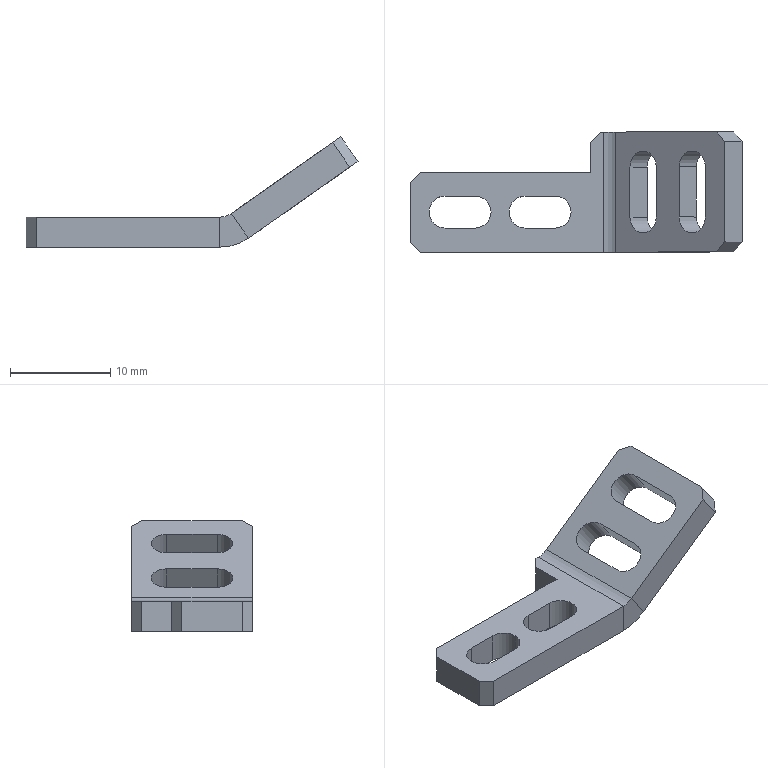Part | SolidWorks | features ICE 2, Chamfer 1, Cut 1, EdgeFlange 1, FlatPattern 1, SMBaseFlange 1, SheetMetal 1 | 1 solid | 39 faces | box 33.189 x 12 x 11.03 mm | volume 781.956 mm3 | plane 27 | cylinder 12 | commonest cylinder face diameters 3.2 x10 4 x1 10 x1
STEP:
#1=CARTESIAN_POINT('',(6.1,-2.,-3.));
#2=VERTEX_POINT('',#1);
#3=CARTESIAN_POINT('',(4.5,-0.4,-3.));
#4=VERTEX_POINT('',#3);
#5=CARTESIAN_POINT('',(4.5,-2.,-3.));
#6=DIRECTION('',(0.,0.,1.));
#7=DIRECTION('',(1.,0.,0.));
#8=AXIS2_PLACEMENT_3D('',#5,#6,#7);
#9=CIRCLE('',#8,1.6);
#10=EDGE_CURVE('',#2,#4,#9,.T.);
#11=ORIENTED_EDGE('',*,*,#10,.F.);
#12=CARTESIAN_POINT('',(6.1,-2.,0.));
#13=VERTEX_POINT('',#12);
#14=CARTESIAN_POINT('',(6.1,-2.,-3.));
#15=DIRECTION('',(0.,0.,1.));
#16=VECTOR('',#15,1000.);
#17=LINE('',#14,#16);
#18=EDGE_CURVE('',#2,#13,#17,.T.);
#19=ORIENTED_EDGE('',*,*,#18,.T.);
#20=CARTESIAN_POINT('',(4.5,-0.4,0.));
#21=VERTEX_POINT('',#20);
#22=CARTESIAN_POINT('',(4.5,-2.,0.));
#23=DIRECTION('',(0.,0.,1.));
#24=DIRECTION('',(1.,0.,0.));
#25=AXIS2_PLACEMENT_3D('',#22,#23,#24);
#26=CIRCLE('',#25,1.6);
#27=EDGE_CURVE('',#13,#21,#26,.T.);
#28=ORIENTED_EDGE('',*,*,#27,.T.);
#29=CARTESIAN_POINT('',(4.5,-0.4,-3.));
#30=DIRECTION('',(0.,0.,1.));
#31=VECTOR('',#30,1000.);
#32=LINE('',#29,#31);
#33=EDGE_CURVE('',#4,#21,#32,.T.);
#34=ORIENTED_EDGE('',*,*,#33,.F.);
#35=EDGE_LOOP('',(#11,#19,#28,#34));
#36=FACE_OUTER_BOUND('',#35,.T.);
#37=CARTESIAN_POINT('',(4.5,-2.,-3.));
#38=DIRECTION('',(0.,0.,1.));
#39=DIRECTION('',(1.,0.,0.));
#40=AXIS2_PLACEMENT_3D('',#37,#38,#39);
#41=CYLINDRICAL_SURFACE('',#40,1.6);
#42=ADVANCED_FACE('',(#36),#41,.F.);
#43=CARTESIAN_POINT('',(-1.9,-2.,-3.));
#44=VERTEX_POINT('',#43);
#45=CARTESIAN_POINT('',(-3.5,-0.4,-3.));
#46=VERTEX_POINT('',#45);
#47=CARTESIAN_POINT('',(-3.5,-2.,-3.));
#48=DIRECTION('',(0.,0.,1.));
#49=DIRECTION('',(1.,0.,0.));
#50=AXIS2_PLACEMENT_3D('',#47,#48,#49);
#51=CIRCLE('',#50,1.6);
#52=EDGE_CURVE('',#44,#46,#51,.T.);
#53=ORIENTED_EDGE('',*,*,#52,.F.);
#54=CARTESIAN_POINT('',(-1.9,-2.,0.));
#55=VERTEX_POINT('',#54);
#56=CARTESIAN_POINT('',(-1.9,-2.,-3.));
#57=DIRECTION('',(0.,0.,1.));
#58=VECTOR('',#57,1000.);
#59=LINE('',#56,#58);
#60=EDGE_CURVE('',#44,#55,#59,.T.);
#61=ORIENTED_EDGE('',*,*,#60,.T.);
#62=CARTESIAN_POINT('',(-3.5,-0.4,0.));
#63=VERTEX_POINT('',#62);
#64=CARTESIAN_POINT('',(-3.5,-2.,0.));
#65=DIRECTION('',(0.,0.,1.));
#66=DIRECTION('',(1.,0.,0.));
#67=AXIS2_PLACEMENT_3D('',#64,#65,#66);
#68=CIRCLE('',#67,1.6);
#69=EDGE_CURVE('',#55,#63,#68,.T.);
#70=ORIENTED_EDGE('',*,*,#69,.T.);
#71=CARTESIAN_POINT('',(-3.5,-0.4,-3.));
#72=DIRECTION('',(0.,0.,1.));
#73=VECTOR('',#72,1000.);
#74=LINE('',#71,#73);
#75=EDGE_CURVE('',#46,#63,#74,.T.);
#76=ORIENTED_EDGE('',*,*,#75,.F.);
#77=EDGE_LOOP('',(#53,#61,#70,#76));
#78=FACE_OUTER_BOUND('',#77,.T.);
#79=CARTESIAN_POINT('',(-3.5,-2.,-3.));
#80=DIRECTION('',(0.,0.,1.));
#81=DIRECTION('',(1.,0.,0.));
#82=AXIS2_PLACEMENT_3D('',#79,#80,#81);
#83=CYLINDRICAL_SURFACE('',#82,1.6);
#84=ADVANCED_FACE('',(#78),#83,.F.);
#85=CARTESIAN_POINT('',(9.369,6.,-3.));
#86=VERTEX_POINT('',#85);
#87=CARTESIAN_POINT('',(9.,6.,-3.));
#88=VERTEX_POINT('',#87);
#89=CARTESIAN_POINT('',(-10.,6.,-3.));
#90=DIRECTION('',(-1.,0.,0.));
#91=VECTOR('',#90,1000.);
#92=LINE('',#89,#91);
#93=EDGE_CURVE('',#86,#88,#92,.T.);
#94=ORIENTED_EDGE('',*,*,#93,.T.);
#95=CARTESIAN_POINT('',(9.,6.,0.));
#96=VERTEX_POINT('',#95);
#97=CARTESIAN_POINT('',(9.,6.,0.));
#98=DIRECTION('',(0.,0.,1.));
#99=VECTOR('',#98,1000.);
#100=LINE('',#97,#99);
#101=EDGE_CURVE('',#88,#96,#100,.T.);
#102=ORIENTED_EDGE('',*,*,#101,.T.);
#103=CARTESIAN_POINT('',(9.369,6.,0.));
#104=VERTEX_POINT('',#103);
#105=CARTESIAN_POINT('',(-10.,6.,0.));
#106=DIRECTION('',(-1.,0.,0.));
#107=VECTOR('',#106,1000.);
#108=LINE('',#105,#107);
#109=EDGE_CURVE('',#104,#96,#108,.T.);
#110=ORIENTED_EDGE('',*,*,#109,.F.);
#111=CARTESIAN_POINT('',(9.369,6.,0.));
#112=DIRECTION('',(0.,0.,-1.));
#113=VECTOR('',#112,1000.);
#114=LINE('',#111,#113);
#115=EDGE_CURVE('',#104,#86,#114,.T.);
#116=ORIENTED_EDGE('',*,*,#115,.T.);
#117=EDGE_LOOP('',(#94,#102,#110,#116));
#118=FACE_OUTER_BOUND('',#117,.T.);
#119=CARTESIAN_POINT('',(-10.,6.,-3.));
#120=DIRECTION('',(0.,1.,0.));
#121=DIRECTION('',(0.,0.,1.));
#122=AXIS2_PLACEMENT_3D('',#119,#120,#121);
#123=PLANE('',#122);
#124=ADVANCED_FACE('',(#118),#123,.T.);
#125=CARTESIAN_POINT('',(1.5,-0.4,-3.));
#126=VERTEX_POINT('',#125);
#127=CARTESIAN_POINT('',(1.5,-0.4,-3.));
#128=DIRECTION('',(-1.,0.,0.));
#129=VECTOR('',#128,1000.);
#130=LINE('',#127,#129);
#131=EDGE_CURVE('',#4,#126,#130,.T.);
#132=ORIENTED_EDGE('',*,*,#131,.T.);
#133=CARTESIAN_POINT('',(1.5,-3.6,-3.));
#134=VERTEX_POINT('',#133);
#135=CARTESIAN_POINT('',(1.5,-2.,-3.));
#136=DIRECTION('',(0.,0.,1.));
#137=DIRECTION('',(1.,0.,0.));
#138=AXIS2_PLACEMENT_3D('',#135,#136,#137);
#139=CIRCLE('',#138,1.6);
#140=EDGE_CURVE('',#126,#134,#139,.T.);
#141=ORIENTED_EDGE('',*,*,#140,.T.);
#142=CARTESIAN_POINT('',(4.5,-3.6,-3.));
#143=VERTEX_POINT('',#142);
#144=CARTESIAN_POINT('',(1.5,-3.6,-3.));
#145=DIRECTION('',(1.,0.,0.));
#146=VECTOR('',#145,1000.);
#147=LINE('',#144,#146);
#148=EDGE_CURVE('',#134,#143,#147,.T.);
#149=ORIENTED_EDGE('',*,*,#148,.T.);
#150=CARTESIAN_POINT('',(4.5,-2.,-3.));
#151=DIRECTION('',(0.,0.,1.));
#152=DIRECTION('',(1.,0.,0.));
#153=AXIS2_PLACEMENT_3D('',#150,#151,#152);
#154=CIRCLE('',#153,1.6);
#155=EDGE_CURVE('',#143,#2,#154,.T.);
#156=ORIENTED_EDGE('',*,*,#155,.T.);
#157=ORIENTED_EDGE('',*,*,#10,.T.);
#158=EDGE_LOOP('',(#132,#141,#149,#156,#157));
#159=FACE_BOUND('',#158,.T.);
#160=CARTESIAN_POINT('',(-6.5,-0.4,-3.));
#161=VERTEX_POINT('',#160);
#162=CARTESIAN_POINT('',(-6.5,-0.4,-3.));
#163=DIRECTION('',(-1.,0.,0.));
#164=VECTOR('',#163,1000.);
#165=LINE('',#162,#164);
#166=EDGE_CURVE('',#46,#161,#165,.T.);
#167=ORIENTED_EDGE('',*,*,#166,.T.);
#168=CARTESIAN_POINT('',(-6.5,-3.6,-3.));
#169=VERTEX_POINT('',#168);
#170=CARTESIAN_POINT('',(-6.5,-2.,-3.));
#171=DIRECTION('',(0.,0.,1.));
#172=DIRECTION('',(1.,0.,0.));
#173=AXIS2_PLACEMENT_3D('',#170,#171,#172);
#174=CIRCLE('',#173,1.6);
#175=EDGE_CURVE('',#161,#169,#174,.T.);
#176=ORIENTED_EDGE('',*,*,#175,.T.);
#177=CARTESIAN_POINT('',(-3.5,-3.6,-3.));
#178=VERTEX_POINT('',#177);
#179=CARTESIAN_POINT('',(-6.5,-3.6,-3.));
#180=DIRECTION('',(1.,0.,0.));
#181=VECTOR('',#180,1000.);
#182=LINE('',#179,#181);
#183=EDGE_CURVE('',#169,#178,#182,.T.);
#184=ORIENTED_EDGE('',*,*,#183,.T.);
#185=CARTESIAN_POINT('',(-3.5,-2.,-3.));
#186=DIRECTION('',(0.,0.,1.));
#187=DIRECTION('',(1.,0.,0.));
#188=AXIS2_PLACEMENT_3D('',#185,#186,#187);
#189=CIRCLE('',#188,1.6);
#190=EDGE_CURVE('',#178,#44,#189,.T.);
#191=ORIENTED_EDGE('',*,*,#190,.T.);
#192=ORIENTED_EDGE('',*,*,#52,.T.);
#193=EDGE_LOOP('',(#167,#176,#184,#191,#192));
#194=FACE_BOUND('',#193,.T.);
#195=CARTESIAN_POINT('',(8.,2.,-3.));
#196=VERTEX_POINT('',#195);
#197=CARTESIAN_POINT('',(8.,5.,-3.));
#198=VERTEX_POINT('',#197);
#199=CARTESIAN_POINT('',(8.,6.,-3.));
#200=DIRECTION('',(0.,1.,0.));
#201=VECTOR('',#200,1000.);
#202=LINE('',#199,#201);
#203=EDGE_CURVE('',#196,#198,#202,.T.);
#204=ORIENTED_EDGE('',*,*,#203,.T.);
#205=CARTESIAN_POINT('',(9.,6.,-3.));
#206=DIRECTION('',(0.7071,0.7071,0.));
#207=VECTOR('',#206,1000.);
#208=LINE('',#205,#207);
#209=EDGE_CURVE('',#198,#88,#208,.T.);
#210=ORIENTED_EDGE('',*,*,#209,.T.);
#211=ORIENTED_EDGE('',*,*,#93,.F.);
#212=CARTESIAN_POINT('',(9.369,-6.,-3.));
#213=VERTEX_POINT('',#212);
#214=CARTESIAN_POINT('',(9.369,6.,-3.));
#215=DIRECTION('',(0.,-1.,0.));
#216=VECTOR('',#215,1000.);
#217=LINE('',#214,#216);
#218=EDGE_CURVE('',#86,#213,#217,.T.);
#219=ORIENTED_EDGE('',*,*,#218,.T.);
#220=CARTESIAN_POINT('',(-9.,-6.,-3.));
#221=VERTEX_POINT('',#220);
#222=CARTESIAN_POINT('',(-10.,-6.,-3.));
#223=DIRECTION('',(1.,0.,0.));
#224=VECTOR('',#223,1000.);
#225=LINE('',#222,#224);
#226=EDGE_CURVE('',#221,#213,#225,.T.);
#227=ORIENTED_EDGE('',*,*,#226,.F.);
#228=CARTESIAN_POINT('',(-10.,-5.,-3.));
#229=VERTEX_POINT('',#228);
#230=CARTESIAN_POINT('',(-10.,-5.,-3.));
#231=DIRECTION('',(-0.7071,0.7071,0.));
#232=VECTOR('',#231,1000.);
#233=LINE('',#230,#232);
#234=EDGE_CURVE('',#221,#229,#233,.T.);
#235=ORIENTED_EDGE('',*,*,#234,.T.);
#236=CARTESIAN_POINT('',(-10.,1.,-3.));
#237=VERTEX_POINT('',#236);
#238=CARTESIAN_POINT('',(-10.,6.,-3.));
#239=DIRECTION('',(0.,-1.,0.));
#240=VECTOR('',#239,1000.);
#241=LINE('',#238,#240);
#242=EDGE_CURVE('',#237,#229,#241,.T.);
#243=ORIENTED_EDGE('',*,*,#242,.F.);
#244=CARTESIAN_POINT('',(-9.,2.,-3.));
#245=VERTEX_POINT('',#244);
#246=CARTESIAN_POINT('',(-9.,2.,-3.));
#247=DIRECTION('',(0.7071,0.7071,0.));
#248=VECTOR('',#247,1000.);
#249=LINE('',#246,#248);
#250=EDGE_CURVE('',#237,#245,#249,.T.);
#251=ORIENTED_EDGE('',*,*,#250,.T.);
#252=CARTESIAN_POINT('',(-10.,2.,-3.));
#253=DIRECTION('',(1.,0.,0.));
#254=VECTOR('',#253,1000.);
#255=LINE('',#252,#254);
#256=EDGE_CURVE('',#245,#196,#255,.T.);
#257=ORIENTED_EDGE('',*,*,#256,.T.);
#258=EDGE_LOOP('',(#204,#210,#211,#219,#227,#235,#243,#251,#257));
#259=FACE_OUTER_BOUND('',#258,.T.);
#260=CARTESIAN_POINT('',(0.,0.,-3.));
#261=DIRECTION('',(0.,0.,1.));
#262=DIRECTION('',(1.,0.,0.));
#263=AXIS2_PLACEMENT_3D('',#260,#261,#262);
#264=PLANE('',#263);
#265=ADVANCED_FACE('',(#159,#194,#259),#264,.F.);
#266=ORIENTED_EDGE('',*,*,#109,.T.);
#267=CARTESIAN_POINT('',(8.,5.,0.));
#268=VERTEX_POINT('',#267);
#269=CARTESIAN_POINT('',(1.5,-1.5,0.));
#270=DIRECTION('',(-0.7071,-0.7071,0.));
#271=VECTOR('',#270,1000.);
#272=LINE('',#269,#271);
#273=EDGE_CURVE('',#96,#268,#272,.T.);
#274=ORIENTED_EDGE('',*,*,#273,.T.);
#275=CARTESIAN_POINT('',(8.,2.,0.));
#276=VERTEX_POINT('',#275);
#277=CARTESIAN_POINT('',(8.,6.,0.));
#278=DIRECTION('',(0.,1.,0.));
#279=VECTOR('',#278,1000.);
#280=LINE('',#277,#279);
#281=EDGE_CURVE('',#276,#268,#280,.T.);
#282=ORIENTED_EDGE('',*,*,#281,.F.);
#283=CARTESIAN_POINT('',(-9.,2.,0.));
#284=VERTEX_POINT('',#283);
#285=CARTESIAN_POINT('',(-10.,2.,0.));
#286=DIRECTION('',(1.,0.,0.));
#287=VECTOR('',#286,1000.);
#288=LINE('',#285,#287);
#289=EDGE_CURVE('',#284,#276,#288,.T.);
#290=ORIENTED_EDGE('',*,*,#289,.F.);
#291=CARTESIAN_POINT('',(-10.,1.,0.));
#292=VERTEX_POINT('',#291);
#293=CARTESIAN_POINT('',(-5.5,5.5,0.));
#294=DIRECTION('',(-0.7071,-0.7071,0.));
#295=VECTOR('',#294,1000.);
#296=LINE('',#293,#295);
#297=EDGE_CURVE('',#284,#292,#296,.T.);
#298=ORIENTED_EDGE('',*,*,#297,.T.);
#299=CARTESIAN_POINT('',(-10.,-5.,0.));
#300=VERTEX_POINT('',#299);
#301=CARTESIAN_POINT('',(-10.,6.,0.));
#302=DIRECTION('',(0.,-1.,0.));
#303=VECTOR('',#302,1000.);
#304=LINE('',#301,#303);
#305=EDGE_CURVE('',#292,#300,#304,.T.);
#306=ORIENTED_EDGE('',*,*,#305,.T.);
#307=CARTESIAN_POINT('',(-9.,-6.,0.));
#308=VERTEX_POINT('',#307);
#309=CARTESIAN_POINT('',(-7.5,-7.5,0.));
#310=DIRECTION('',(0.7071,-0.7071,0.));
#311=VECTOR('',#310,1000.);
#312=LINE('',#309,#311);
#313=EDGE_CURVE('',#300,#308,#312,.T.);
#314=ORIENTED_EDGE('',*,*,#313,.T.);
#315=CARTESIAN_POINT('',(9.369,-6.,0.));
#316=VERTEX_POINT('',#315);
#317=CARTESIAN_POINT('',(-10.,-6.,0.));
#318=DIRECTION('',(1.,0.,0.));
#319=VECTOR('',#318,1000.);
#320=LINE('',#317,#319);
#321=EDGE_CURVE('',#308,#316,#320,.T.);
#322=ORIENTED_EDGE('',*,*,#321,.T.);
#323=CARTESIAN_POINT('',(9.369,6.,0.));
#324=DIRECTION('',(0.,-1.,0.));
#325=VECTOR('',#324,1000.);
#326=LINE('',#323,#325);
#327=EDGE_CURVE('',#104,#316,#326,.T.);
#328=ORIENTED_EDGE('',*,*,#327,.F.);
#329=EDGE_LOOP('',(#266,#274,#282,#290,#298,#306,#314,#322,#328));
#330=FACE_OUTER_BOUND('',#329,.T.);
#331=CARTESIAN_POINT('',(1.5,-0.4,0.));
#332=VERTEX_POINT('',#331);
#333=CARTESIAN_POINT('',(1.5,-3.6,0.));
#334=VERTEX_POINT('',#333);
#335=CARTESIAN_POINT('',(1.5,-2.,0.));
#336=DIRECTION('',(0.,0.,1.));
#337=DIRECTION('',(1.,0.,0.));
#338=AXIS2_PLACEMENT_3D('',#335,#336,#337);
#339=CIRCLE('',#338,1.6);
#340=EDGE_CURVE('',#332,#334,#339,.T.);
#341=ORIENTED_EDGE('',*,*,#340,.F.);
#342=CARTESIAN_POINT('',(1.5,-0.4,0.));
#343=DIRECTION('',(-1.,0.,0.));
#344=VECTOR('',#343,1000.);
#345=LINE('',#342,#344);
#346=EDGE_CURVE('',#21,#332,#345,.T.);
#347=ORIENTED_EDGE('',*,*,#346,.F.);
#348=ORIENTED_EDGE('',*,*,#27,.F.);
#349=CARTESIAN_POINT('',(4.5,-3.6,0.));
#350=VERTEX_POINT('',#349);
#351=CARTESIAN_POINT('',(4.5,-2.,0.));
#352=DIRECTION('',(0.,0.,1.));
#353=DIRECTION('',(1.,0.,0.));
#354=AXIS2_PLACEMENT_3D('',#351,#352,#353);
#355=CIRCLE('',#354,1.6);
#356=EDGE_CURVE('',#350,#13,#355,.T.);
#357=ORIENTED_EDGE('',*,*,#356,.F.);
#358=CARTESIAN_POINT('',(1.5,-3.6,0.));
#359=DIRECTION('',(1.,0.,0.));
#360=VECTOR('',#359,1000.);
#361=LINE('',#358,#360);
#362=EDGE_CURVE('',#334,#350,#361,.T.);
#363=ORIENTED_EDGE('',*,*,#362,.F.);
#364=EDGE_LOOP('',(#341,#347,#348,#357,#363));
#365=FACE_BOUND('',#364,.T.);
#366=CARTESIAN_POINT('',(-6.5,-0.4,0.));
#367=VERTEX_POINT('',#366);
#368=CARTESIAN_POINT('',(-6.5,-3.6,0.));
#369=VERTEX_POINT('',#368);
#370=CARTESIAN_POINT('',(-6.5,-2.,0.));
#371=DIRECTION('',(0.,0.,1.));
#372=DIRECTION('',(1.,0.,0.));
#373=AXIS2_PLACEMENT_3D('',#370,#371,#372);
#374=CIRCLE('',#373,1.6);
#375=EDGE_CURVE('',#367,#369,#374,.T.);
#376=ORIENTED_EDGE('',*,*,#375,.F.);
#377=CARTESIAN_POINT('',(-6.5,-0.4,0.));
#378=DIRECTION('',(-1.,0.,0.));
#379=VECTOR('',#378,1000.);
#380=LINE('',#377,#379);
#381=EDGE_CURVE('',#63,#367,#380,.T.);
#382=ORIENTED_EDGE('',*,*,#381,.F.);
#383=ORIENTED_EDGE('',*,*,#69,.F.);
#384=CARTESIAN_POINT('',(-3.5,-3.6,0.));
#385=VERTEX_POINT('',#384);
#386=CARTESIAN_POINT('',(-3.5,-2.,0.));
#387=DIRECTION('',(0.,0.,1.));
#388=DIRECTION('',(1.,0.,0.));
#389=AXIS2_PLACEMENT_3D('',#386,#387,#388);
#390=CIRCLE('',#389,1.6);
#391=EDGE_CURVE('',#385,#55,#390,.T.);
#392=ORIENTED_EDGE('',*,*,#391,.F.);
#393=CARTESIAN_POINT('',(-6.5,-3.6,0.));
#394=DIRECTION('',(1.,0.,0.));
#395=VECTOR('',#394,1000.);
#396=LINE('',#393,#395);
#397=EDGE_CURVE('',#369,#385,#396,.T.);
#398=ORIENTED_EDGE('',*,*,#397,.F.);
#399=EDGE_LOOP('',(#376,#382,#383,#392,#398));
#400=FACE_BOUND('',#399,.T.);
#401=CARTESIAN_POINT('',(0.,0.,0.));
#402=DIRECTION('',(0.,0.,1.));
#403=DIRECTION('',(1.,0.,0.));
#404=AXIS2_PLACEMENT_3D('',#401,#402,#403);
#405=PLANE('',#404);
#406=ADVANCED_FACE('',(#330,#365,#400),#405,.T.);
#407=ORIENTED_EDGE('',*,*,#321,.F.);
#408=CARTESIAN_POINT('',(-9.,-6.,-3.));
#409=DIRECTION('',(0.,0.,-1.));
#410=VECTOR('',#409,1000.);
#411=LINE('',#408,#410);
#412=EDGE_CURVE('',#308,#221,#411,.T.);
#413=ORIENTED_EDGE('',*,*,#412,.T.);
#414=ORIENTED_EDGE('',*,*,#226,.T.);
#415=CARTESIAN_POINT('',(9.369,-6.,0.));
#416=DIRECTION('',(0.,0.,-1.));
#417=VECTOR('',#416,1000.);
#418=LINE('',#415,#417);
#419=EDGE_CURVE('',#316,#213,#418,.T.);
#420=ORIENTED_EDGE('',*,*,#419,.F.);
#421=EDGE_LOOP('',(#407,#413,#414,#420));
#422=FACE_OUTER_BOUND('',#421,.T.);
#423=CARTESIAN_POINT('',(-10.,-6.,-3.));
#424=DIRECTION('',(0.,-1.,0.));
#425=DIRECTION('',(0.,0.,-1.));
#426=AXIS2_PLACEMENT_3D('',#423,#424,#425);
#427=PLANE('',#426);
#428=ADVANCED_FACE('',(#422),#427,.T.);
#429=ORIENTED_EDGE('',*,*,#242,.T.);
#430=CARTESIAN_POINT('',(-10.,-5.,-3.));
#431=DIRECTION('',(0.,0.,1.));
#432=VECTOR('',#431,1000.);
#433=LINE('',#430,#432);
#434=EDGE_CURVE('',#229,#300,#433,.T.);
#435=ORIENTED_EDGE('',*,*,#434,.T.);
#436=ORIENTED_EDGE('',*,*,#305,.F.);
#437=CARTESIAN_POINT('',(-10.,1.,-3.));
#438=DIRECTION('',(0.,0.,-1.));
#439=VECTOR('',#438,1000.);
#440=LINE('',#437,#439);
#441=EDGE_CURVE('',#292,#237,#440,.T.);
#442=ORIENTED_EDGE('',*,*,#441,.T.);
#443=EDGE_LOOP('',(#429,#435,#436,#442));
#444=FACE_OUTER_BOUND('',#443,.T.);
#445=CARTESIAN_POINT('',(-10.,6.,-3.));
#446=DIRECTION('',(-1.,0.,0.));
#447=DIRECTION('',(0.,0.,1.));
#448=AXIS2_PLACEMENT_3D('',#445,#446,#447);
#449=PLANE('',#448);
#450=ADVANCED_FACE('',(#444),#449,.T.);
#451=CARTESIAN_POINT('',(10.517,-6.,0.3617));
#452=VERTEX_POINT('',#451);
#453=CARTESIAN_POINT('',(12.237,-6.,-2.096));
#454=VERTEX_POINT('',#453);
#455=CARTESIAN_POINT('',(10.517,-6.,0.3617));
#456=DIRECTION('',(0.5736,0.,-0.8192));
#457=VECTOR('',#456,1000.);
#458=LINE('',#455,#457);
#459=EDGE_CURVE('',#452,#454,#458,.T.);
#460=ORIENTED_EDGE('',*,*,#459,.F.);
#461=CARTESIAN_POINT('',(9.369,-6.,2.));
#462=DIRECTION('',(0.,-1.,0.));
#463=DIRECTION('',(0.,0.,1.));
#464=AXIS2_PLACEMENT_3D('',#461,#462,#463);
#465=CIRCLE('',#464,2.);
#466=EDGE_CURVE('',#316,#452,#465,.T.);
#467=ORIENTED_EDGE('',*,*,#466,.F.);
#468=ORIENTED_EDGE('',*,*,#419,.T.);
#469=CARTESIAN_POINT('',(9.369,-6.,2.));
#470=DIRECTION('',(0.,-1.,0.));
#471=DIRECTION('',(0.,0.,1.));
#472=AXIS2_PLACEMENT_3D('',#469,#470,#471);
#473=CIRCLE('',#472,5.);
#474=EDGE_CURVE('',#213,#454,#473,.T.);
#475=ORIENTED_EDGE('',*,*,#474,.T.);
#476=EDGE_LOOP('',(#460,#467,#468,#475));
#477=FACE_OUTER_BOUND('',#476,.T.);
#478=CARTESIAN_POINT('',(9.369,-6.,2.));
#479=DIRECTION('',(0.,-1.,0.));
#480=DIRECTION('',(0.,0.,-1.));
#481=AXIS2_PLACEMENT_3D('',#478,#479,#480);
#482=PLANE('',#481);
#483=ADVANCED_FACE('',(#477),#482,.T.);
#484=CARTESIAN_POINT('',(10.517,6.,0.3617));
#485=VERTEX_POINT('',#484);
#486=CARTESIAN_POINT('',(9.369,6.,2.));
#487=DIRECTION('',(0.,1.,0.));
#488=DIRECTION('',(0.,0.,1.));
#489=AXIS2_PLACEMENT_3D('',#486,#487,#488);
#490=CIRCLE('',#489,2.);
#491=EDGE_CURVE('',#485,#104,#490,.T.);
#492=ORIENTED_EDGE('',*,*,#491,.F.);
#493=CARTESIAN_POINT('',(12.237,6.,-2.096));
#494=VERTEX_POINT('',#493);
#495=CARTESIAN_POINT('',(10.517,6.,0.3617));
#496=DIRECTION('',(0.5736,0.,-0.8192));
#497=VECTOR('',#496,1000.);
#498=LINE('',#495,#497);
#499=EDGE_CURVE('',#485,#494,#498,.T.);
#500=ORIENTED_EDGE('',*,*,#499,.T.);
#501=CARTESIAN_POINT('',(9.369,6.,2.));
#502=DIRECTION('',(0.,1.,0.));
#503=DIRECTION('',(0.,0.,1.));
#504=AXIS2_PLACEMENT_3D('',#501,#502,#503);
#505=CIRCLE('',#504,5.);
#506=EDGE_CURVE('',#494,#86,#505,.T.);
#507=ORIENTED_EDGE('',*,*,#506,.T.);
#508=ORIENTED_EDGE('',*,*,#115,.F.);
#509=EDGE_LOOP('',(#492,#500,#507,#508));
#510=FACE_OUTER_BOUND('',#509,.T.);
#511=CARTESIAN_POINT('',(9.369,6.,2.));
#512=DIRECTION('',(0.,-1.,0.));
#513=DIRECTION('',(0.,0.,-1.));
#514=AXIS2_PLACEMENT_3D('',#511,#512,#513);
#515=PLANE('',#514);
#516=ADVANCED_FACE('',(#510),#515,.F.);
#517=ORIENTED_EDGE('',*,*,#218,.F.);
#518=ORIENTED_EDGE('',*,*,#506,.F.);
#519=CARTESIAN_POINT('',(12.237,0.,-2.096));
#520=DIRECTION('',(0.,1.,0.));
#521=VECTOR('',#520,1000.);
#522=LINE('',#519,#521);
#523=EDGE_CURVE('',#454,#494,#522,.T.);
#524=ORIENTED_EDGE('',*,*,#523,.F.);
#525=ORIENTED_EDGE('',*,*,#474,.F.);
#526=EDGE_LOOP('',(#517,#518,#524,#525));
#527=FACE_OUTER_BOUND('',#526,.T.);
#528=CARTESIAN_POINT('',(9.369,6.,2.));
#529=DIRECTION('',(0.,1.,0.));
#530=DIRECTION('',(0.5736,0.,-0.8192));
#531=AXIS2_PLACEMENT_3D('',#528,#529,#530);
#532=CYLINDRICAL_SURFACE('',#531,5.);
#533=ADVANCED_FACE('',(#527),#532,.T.);
#534=ORIENTED_EDGE('',*,*,#327,.T.);
#535=ORIENTED_EDGE('',*,*,#466,.T.);
#536=CARTESIAN_POINT('',(10.517,-6.,0.3617));
#537=DIRECTION('',(0.,1.,0.));
#538=VECTOR('',#537,1000.);
#539=LINE('',#536,#538);
#540=EDGE_CURVE('',#452,#485,#539,.T.);
#541=ORIENTED_EDGE('',*,*,#540,.T.);
#542=ORIENTED_EDGE('',*,*,#491,.T.);
#543=EDGE_LOOP('',(#534,#535,#541,#542));
#544=FACE_OUTER_BOUND('',#543,.T.);
#545=CARTESIAN_POINT('',(9.369,6.,2.));
#546=DIRECTION('',(0.,1.,0.));
#547=DIRECTION('',(0.5736,0.,-0.8192));
#548=AXIS2_PLACEMENT_3D('',#545,#546,#547);
#549=CYLINDRICAL_SURFACE('',#548,2.);
#550=ADVANCED_FACE('',(#544),#549,.F.);
#551=CARTESIAN_POINT('',(20.649,6.,7.456));
#552=VERTEX_POINT('',#551);
#553=CARTESIAN_POINT('',(10.,6.,0.));
#554=DIRECTION('',(-0.8192,0.,-0.5736));
#555=VECTOR('',#554,1000.);
#556=LINE('',#553,#555);
#557=EDGE_CURVE('',#552,#485,#556,.T.);
#558=ORIENTED_EDGE('',*,*,#557,.F.);
#559=CARTESIAN_POINT('',(22.37,6.,4.999));
#560=VERTEX_POINT('',#559);
#561=CARTESIAN_POINT('',(22.37,6.,4.999));
#562=DIRECTION('',(0.5736,0.,-0.8192));
#563=VECTOR('',#562,1000.);
#564=LINE('',#561,#563);
#565=EDGE_CURVE('',#552,#560,#564,.T.);
#566=ORIENTED_EDGE('',*,*,#565,.T.);
#567=CARTESIAN_POINT('',(11.721,6.,-2.457));
#568=DIRECTION('',(-0.8192,0.,-0.5736));
#569=VECTOR('',#568,1000.);
#570=LINE('',#567,#569);
#571=EDGE_CURVE('',#560,#494,#570,.T.);
#572=ORIENTED_EDGE('',*,*,#571,.T.);
#573=ORIENTED_EDGE('',*,*,#499,.F.);
#574=EDGE_LOOP('',(#558,#566,#572,#573));
#575=FACE_OUTER_BOUND('',#574,.T.);
#576=CARTESIAN_POINT('',(11.721,6.,-2.457));
#577=DIRECTION('',(0.,1.,0.));
#578=DIRECTION('',(-1.,0.,0.));
#579=AXIS2_PLACEMENT_3D('',#576,#577,#578);
#580=PLANE('',#579);
#581=ADVANCED_FACE('',(#575),#580,.T.);
#582=CARTESIAN_POINT('',(22.37,-6.,4.999));
#583=VERTEX_POINT('',#582);
#584=CARTESIAN_POINT('',(23.189,-6.,5.573));
#585=DIRECTION('',(0.8192,0.,0.5736));
#586=VECTOR('',#585,1000.);
#587=LINE('',#584,#586);
#588=EDGE_CURVE('',#454,#583,#587,.T.);
#589=ORIENTED_EDGE('',*,*,#588,.T.);
#590=CARTESIAN_POINT('',(20.649,-6.,7.456));
#591=VERTEX_POINT('',#590);
#592=CARTESIAN_POINT('',(22.37,-6.,4.999));
#593=DIRECTION('',(-0.5736,0.,0.8192));
#594=VECTOR('',#593,1000.);
#595=LINE('',#592,#594);
#596=EDGE_CURVE('',#583,#591,#595,.T.);
#597=ORIENTED_EDGE('',*,*,#596,.T.);
#598=CARTESIAN_POINT('',(21.468,-6.,8.03));
#599=DIRECTION('',(0.8192,0.,0.5736));
#600=VECTOR('',#599,1000.);
#601=LINE('',#598,#600);
#602=EDGE_CURVE('',#452,#591,#601,.T.);
#603=ORIENTED_EDGE('',*,*,#602,.F.);
#604=ORIENTED_EDGE('',*,*,#459,.T.);
#605=EDGE_LOOP('',(#589,#597,#603,#604));
#606=FACE_OUTER_BOUND('',#605,.T.);
#607=CARTESIAN_POINT('',(23.189,-6.,5.573));
#608=DIRECTION('',(0.,-1.,0.));
#609=DIRECTION('',(1.,0.,0.));
#610=AXIS2_PLACEMENT_3D('',#607,#608,#609);
#611=PLANE('',#610);
#612=ADVANCED_FACE('',(#606),#611,.T.);
#613=CARTESIAN_POINT('',(18.625,2.5,2.377));
#614=VERTEX_POINT('',#613);
#615=CARTESIAN_POINT('',(21.246,2.5,4.212));
#616=VERTEX_POINT('',#615);
#617=CARTESIAN_POINT('',(19.935,2.5,3.294));
#618=DIRECTION('',(0.5736,0.,-0.8192));
#619=DIRECTION('',(-0.8192,0.,-0.5736));
#620=AXIS2_PLACEMENT_3D('',#617,#618,#619);
#621=CIRCLE('',#620,1.6);
#622=EDGE_CURVE('',#614,#616,#621,.T.);
#623=ORIENTED_EDGE('',*,*,#622,.F.);
#624=CARTESIAN_POINT('',(18.625,-2.5,2.377));
#625=VERTEX_POINT('',#624);
#626=CARTESIAN_POINT('',(18.625,0.,2.377));
#627=DIRECTION('',(0.,1.,0.));
#628=VECTOR('',#627,1000.);
#629=LINE('',#626,#628);
#630=EDGE_CURVE('',#625,#614,#629,.T.);
#631=ORIENTED_EDGE('',*,*,#630,.F.);
#632=CARTESIAN_POINT('',(21.246,-2.5,4.212));
#633=VERTEX_POINT('',#632);
#634=CARTESIAN_POINT('',(19.935,-2.5,3.294));
#635=DIRECTION('',(0.5736,0.,-0.8192));
#636=DIRECTION('',(-0.8192,0.,-0.5736));
#637=AXIS2_PLACEMENT_3D('',#634,#635,#636);
#638=CIRCLE('',#637,1.6);
#639=EDGE_CURVE('',#633,#625,#638,.T.);
#640=ORIENTED_EDGE('',*,*,#639,.F.);
#641=CARTESIAN_POINT('',(21.246,0.,4.212));
#642=DIRECTION('',(0.,-1.,0.));
#643=VECTOR('',#642,1000.);
#644=LINE('',#641,#643);
#645=EDGE_CURVE('',#616,#633,#644,.T.);
#646=ORIENTED_EDGE('',*,*,#645,.F.);
#647=EDGE_LOOP('',(#623,#631,#640,#646));
#648=FACE_BOUND('',#647,.T.);
#649=CARTESIAN_POINT('',(13.71,2.5,-1.065));
#650=VERTEX_POINT('',#649);
#651=CARTESIAN_POINT('',(16.331,2.5,0.7707));
#652=VERTEX_POINT('',#651);
#653=CARTESIAN_POINT('',(15.02,2.5,-0.147));
#654=DIRECTION('',(0.5736,0.,-0.8192));
#655=DIRECTION('',(-0.8192,0.,-0.5736));
#656=AXIS2_PLACEMENT_3D('',#653,#654,#655);
#657=CIRCLE('',#656,1.6);
#658=EDGE_CURVE('',#650,#652,#657,.T.);
#659=ORIENTED_EDGE('',*,*,#658,.F.);
#660=CARTESIAN_POINT('',(13.71,-2.5,-1.065));
#661=VERTEX_POINT('',#660);
#662=CARTESIAN_POINT('',(13.71,0.,-1.065));
#663=DIRECTION('',(0.,1.,0.));
#664=VECTOR('',#663,1000.);
#665=LINE('',#662,#664);
#666=EDGE_CURVE('',#661,#650,#665,.T.);
#667=ORIENTED_EDGE('',*,*,#666,.F.);
#668=CARTESIAN_POINT('',(16.331,-2.5,0.7707));
#669=VERTEX_POINT('',#668);
#670=CARTESIAN_POINT('',(15.02,-2.5,-0.147));
#671=DIRECTION('',(0.5736,0.,-0.8192));
#672=DIRECTION('',(-0.8192,0.,-0.5736));
#673=AXIS2_PLACEMENT_3D('',#670,#671,#672);
#674=CIRCLE('',#673,1.6);
#675=EDGE_CURVE('',#669,#661,#674,.T.);
#676=ORIENTED_EDGE('',*,*,#675,.F.);
#677=CARTESIAN_POINT('',(16.331,0.,0.7707));
#678=DIRECTION('',(0.,-1.,0.));
#679=VECTOR('',#678,1000.);
#680=LINE('',#677,#679);
#681=EDGE_CURVE('',#652,#669,#680,.T.);
#682=ORIENTED_EDGE('',*,*,#681,.F.);
#683=EDGE_LOOP('',(#659,#667,#676,#682));
#684=FACE_BOUND('',#683,.T.);
#685=CARTESIAN_POINT('',(23.189,-5.,5.573));
#686=VERTEX_POINT('',#685);
#687=CARTESIAN_POINT('',(23.189,5.,5.573));
#688=VERTEX_POINT('',#687);
#689=CARTESIAN_POINT('',(23.189,6.,5.573));
#690=DIRECTION('',(0.,1.,0.));
#691=VECTOR('',#690,1000.);
#692=LINE('',#689,#691);
#693=EDGE_CURVE('',#686,#688,#692,.T.);
#694=ORIENTED_EDGE('',*,*,#693,.F.);
#695=CARTESIAN_POINT('',(16.148,-13.596,0.6423));
#696=DIRECTION('',(-0.5792,-0.7071,-0.4056));
#697=VECTOR('',#696,1000.);
#698=LINE('',#695,#697);
#699=EDGE_CURVE('',#686,#583,#698,.T.);
#700=ORIENTED_EDGE('',*,*,#699,.T.);
#701=ORIENTED_EDGE('',*,*,#588,.F.);
#702=ORIENTED_EDGE('',*,*,#523,.T.);
#703=ORIENTED_EDGE('',*,*,#571,.F.);
#704=CARTESIAN_POINT('',(16.148,13.596,0.6423));
#705=DIRECTION('',(0.5792,-0.7071,0.4056));
#706=VECTOR('',#705,1000.);
#707=LINE('',#704,#706);
#708=EDGE_CURVE('',#560,#688,#707,.T.);
#709=ORIENTED_EDGE('',*,*,#708,.T.);
#710=EDGE_LOOP('',(#694,#700,#701,#702,#703,#709));
#711=FACE_OUTER_BOUND('',#710,.T.);
#712=CARTESIAN_POINT('',(5.011,0.,-7.156));
#713=DIRECTION('',(0.5736,0.,-0.8192));
#714=DIRECTION('',(-0.8192,0.,-0.5736));
#715=AXIS2_PLACEMENT_3D('',#712,#713,#714);
#716=PLANE('',#715);
#717=ADVANCED_FACE('',(#648,#684,#711),#716,.T.);
#718=CARTESIAN_POINT('',(16.904,2.5,4.834));
#719=VERTEX_POINT('',#718);
#720=CARTESIAN_POINT('',(16.904,-2.5,4.834));
#721=VERTEX_POINT('',#720);
#722=CARTESIAN_POINT('',(16.904,2.5,4.834));
#723=DIRECTION('',(0.,-1.,0.));
#724=VECTOR('',#723,1000.);
#725=LINE('',#722,#724);
#726=EDGE_CURVE('',#719,#721,#725,.T.);
#727=ORIENTED_EDGE('',*,*,#726,.F.);
#728=CARTESIAN_POINT('',(19.525,2.5,6.67));
#729=VERTEX_POINT('',#728);
#730=CARTESIAN_POINT('',(18.215,2.5,5.752));
#731=DIRECTION('',(-0.5736,0.,0.8192));
#732=DIRECTION('',(0.8192,0.,0.5736));
#733=AXIS2_PLACEMENT_3D('',#730,#731,#732);
#734=CIRCLE('',#733,1.6);
#735=EDGE_CURVE('',#729,#719,#734,.T.);
#736=ORIENTED_EDGE('',*,*,#735,.F.);
#737=CARTESIAN_POINT('',(19.525,-2.5,6.67));
#738=VERTEX_POINT('',#737);
#739=CARTESIAN_POINT('',(19.525,2.5,6.67));
#740=DIRECTION('',(0.,1.,0.));
#741=VECTOR('',#740,1000.);
#742=LINE('',#739,#741);
#743=EDGE_CURVE('',#738,#729,#742,.T.);
#744=ORIENTED_EDGE('',*,*,#743,.F.);
#745=CARTESIAN_POINT('',(18.215,-2.5,5.752));
#746=DIRECTION('',(-0.5736,0.,0.8192));
#747=DIRECTION('',(0.8192,0.,0.5736));
#748=AXIS2_PLACEMENT_3D('',#745,#746,#747);
#749=CIRCLE('',#748,1.6);
#750=EDGE_CURVE('',#721,#738,#749,.T.);
#751=ORIENTED_EDGE('',*,*,#750,.F.);
#752=EDGE_LOOP('',(#727,#736,#744,#751));
#753=FACE_BOUND('',#752,.T.);
#754=CARTESIAN_POINT('',(11.989,2.5,1.393));
#755=VERTEX_POINT('',#754);
#756=CARTESIAN_POINT('',(11.989,-2.5,1.393));
#757=VERTEX_POINT('',#756);
#758=CARTESIAN_POINT('',(11.989,2.5,1.393));
#759=DIRECTION('',(0.,-1.,0.));
#760=VECTOR('',#759,1000.);
#761=LINE('',#758,#760);
#762=EDGE_CURVE('',#755,#757,#761,.T.);
#763=ORIENTED_EDGE('',*,*,#762,.F.);
#764=CARTESIAN_POINT('',(14.61,2.5,3.228));
#765=VERTEX_POINT('',#764);
#766=CARTESIAN_POINT('',(13.3,2.5,2.31));
#767=DIRECTION('',(-0.5736,0.,0.8192));
#768=DIRECTION('',(0.8192,0.,0.5736));
#769=AXIS2_PLACEMENT_3D('',#766,#767,#768);
#770=CIRCLE('',#769,1.6);
#771=EDGE_CURVE('',#765,#755,#770,.T.);
#772=ORIENTED_EDGE('',*,*,#771,.F.);
#773=CARTESIAN_POINT('',(14.61,-2.5,3.228));
#774=VERTEX_POINT('',#773);
#775=CARTESIAN_POINT('',(14.61,2.5,3.228));
#776=DIRECTION('',(0.,1.,0.));
#777=VECTOR('',#776,1000.);
#778=LINE('',#775,#777);
#779=EDGE_CURVE('',#774,#765,#778,.T.);
#780=ORIENTED_EDGE('',*,*,#779,.F.);
#781=CARTESIAN_POINT('',(13.3,-2.5,2.31));
#782=DIRECTION('',(-0.5736,0.,0.8192));
#783=DIRECTION('',(0.8192,0.,0.5736));
#784=AXIS2_PLACEMENT_3D('',#781,#782,#783);
#785=CIRCLE('',#784,1.6);
#786=EDGE_CURVE('',#757,#774,#785,.T.);
#787=ORIENTED_EDGE('',*,*,#786,.F.);
#788=EDGE_LOOP('',(#763,#772,#780,#787));
#789=FACE_BOUND('',#788,.T.);
#790=ORIENTED_EDGE('',*,*,#602,.T.);
#791=CARTESIAN_POINT('',(21.468,-5.,8.03));
#792=VERTEX_POINT('',#791);
#793=CARTESIAN_POINT('',(20.649,-6.,7.456));
#794=DIRECTION('',(0.5792,0.7071,0.4056));
#795=VECTOR('',#794,1000.);
#796=LINE('',#793,#795);
#797=EDGE_CURVE('',#591,#792,#796,.T.);
#798=ORIENTED_EDGE('',*,*,#797,.T.);
#799=CARTESIAN_POINT('',(21.468,5.,8.03));
#800=VERTEX_POINT('',#799);
#801=CARTESIAN_POINT('',(21.468,6.,8.03));
#802=DIRECTION('',(0.,1.,0.));
#803=VECTOR('',#802,1000.);
#804=LINE('',#801,#803);
#805=EDGE_CURVE('',#792,#800,#804,.T.);
#806=ORIENTED_EDGE('',*,*,#805,.T.);
#807=CARTESIAN_POINT('',(21.468,5.,8.03));
#808=DIRECTION('',(-0.5792,0.7071,-0.4056));
#809=VECTOR('',#808,1000.);
#810=LINE('',#807,#809);
#811=EDGE_CURVE('',#800,#552,#810,.T.);
#812=ORIENTED_EDGE('',*,*,#811,.T.);
#813=ORIENTED_EDGE('',*,*,#557,.T.);
#814=ORIENTED_EDGE('',*,*,#540,.F.);
#815=EDGE_LOOP('',(#790,#798,#806,#812,#813,#814));
#816=FACE_OUTER_BOUND('',#815,.T.);
#817=CARTESIAN_POINT('',(3.29,0.,-4.698));
#818=DIRECTION('',(0.5736,0.,-0.8192));
#819=DIRECTION('',(-0.8192,0.,-0.5736));
#820=AXIS2_PLACEMENT_3D('',#817,#818,#819);
#821=PLANE('',#820);
#822=ADVANCED_FACE('',(#753,#789,#816),#821,.F.);
#823=ORIENTED_EDGE('',*,*,#805,.F.);
#824=CARTESIAN_POINT('',(23.189,-5.,5.573));
#825=DIRECTION('',(0.5736,0.,-0.8192));
#826=VECTOR('',#825,1000.);
#827=LINE('',#824,#826);
#828=EDGE_CURVE('',#792,#686,#827,.T.);
#829=ORIENTED_EDGE('',*,*,#828,.T.);
#830=ORIENTED_EDGE('',*,*,#693,.T.);
#831=CARTESIAN_POINT('',(23.189,5.,5.573));
#832=DIRECTION('',(-0.5736,0.,0.8192));
#833=VECTOR('',#832,1000.);
#834=LINE('',#831,#833);
#835=EDGE_CURVE('',#688,#800,#834,.T.);
#836=ORIENTED_EDGE('',*,*,#835,.T.);
#837=EDGE_LOOP('',(#823,#829,#830,#836));
#838=FACE_OUTER_BOUND('',#837,.T.);
#839=CARTESIAN_POINT('',(23.189,6.,5.573));
#840=DIRECTION('',(0.8192,0.,0.5736));
#841=DIRECTION('',(0.5736,0.,-0.8192));
#842=AXIS2_PLACEMENT_3D('',#839,#840,#841);
#843=PLANE('',#842);
#844=ADVANCED_FACE('',(#838),#843,.T.);
#845=ORIENTED_EDGE('',*,*,#375,.T.);
#846=CARTESIAN_POINT('',(-6.5,-3.6,-3.));
#847=DIRECTION('',(0.,0.,1.));
#848=VECTOR('',#847,1000.);
#849=LINE('',#846,#848);
#850=EDGE_CURVE('',#169,#369,#849,.T.);
#851=ORIENTED_EDGE('',*,*,#850,.F.);
#852=ORIENTED_EDGE('',*,*,#175,.F.);
#853=CARTESIAN_POINT('',(-6.5,-0.4,-3.));
#854=DIRECTION('',(0.,0.,1.));
#855=VECTOR('',#854,1000.);
#856=LINE('',#853,#855);
#857=EDGE_CURVE('',#161,#367,#856,.T.);
#858=ORIENTED_EDGE('',*,*,#857,.T.);
#859=EDGE_LOOP('',(#845,#851,#852,#858));
#860=FACE_OUTER_BOUND('',#859,.T.);
#861=CARTESIAN_POINT('',(-6.5,-2.,-3.));
#862=DIRECTION('',(0.,0.,1.));
#863=DIRECTION('',(1.,0.,0.));
#864=AXIS2_PLACEMENT_3D('',#861,#862,#863);
#865=CYLINDRICAL_SURFACE('',#864,1.6);
#866=ADVANCED_FACE('',(#860),#865,.F.);
#867=ORIENTED_EDGE('',*,*,#381,.T.);
#868=ORIENTED_EDGE('',*,*,#857,.F.);
#869=ORIENTED_EDGE('',*,*,#166,.F.);
#870=ORIENTED_EDGE('',*,*,#75,.T.);
#871=EDGE_LOOP('',(#867,#868,#869,#870));
#872=FACE_OUTER_BOUND('',#871,.T.);
#873=CARTESIAN_POINT('',(-6.5,-0.4,-3.));
#874=DIRECTION('',(0.,1.,0.));
#875=DIRECTION('',(-1.,0.,0.));
#876=AXIS2_PLACEMENT_3D('',#873,#874,#875);
#877=PLANE('',#876);
#878=ADVANCED_FACE('',(#872),#877,.F.);
#879=ORIENTED_EDGE('',*,*,#60,.F.);
#880=ORIENTED_EDGE('',*,*,#190,.F.);
#881=CARTESIAN_POINT('',(-3.5,-3.6,-3.));
#882=DIRECTION('',(0.,0.,1.));
#883=VECTOR('',#882,1000.);
#884=LINE('',#881,#883);
#885=EDGE_CURVE('',#178,#385,#884,.T.);
#886=ORIENTED_EDGE('',*,*,#885,.T.);
#887=ORIENTED_EDGE('',*,*,#391,.T.);
#888=EDGE_LOOP('',(#879,#880,#886,#887));
#889=FACE_OUTER_BOUND('',#888,.T.);
#890=CARTESIAN_POINT('',(-3.5,-2.,-3.));
#891=DIRECTION('',(0.,0.,1.));
#892=DIRECTION('',(1.,0.,0.));
#893=AXIS2_PLACEMENT_3D('',#890,#891,#892);
#894=CYLINDRICAL_SURFACE('',#893,1.6);
#895=ADVANCED_FACE('',(#889),#894,.F.);
#896=ORIENTED_EDGE('',*,*,#397,.T.);
#897=ORIENTED_EDGE('',*,*,#885,.F.);
#898=ORIENTED_EDGE('',*,*,#183,.F.);
#899=ORIENTED_EDGE('',*,*,#850,.T.);
#900=EDGE_LOOP('',(#896,#897,#898,#899));
#901=FACE_OUTER_BOUND('',#900,.T.);
#902=CARTESIAN_POINT('',(-6.5,-3.6,-3.));
#903=DIRECTION('',(0.,-1.,0.));
#904=DIRECTION('',(1.,0.,0.));
#905=AXIS2_PLACEMENT_3D('',#902,#903,#904);
#906=PLANE('',#905);
#907=ADVANCED_FACE('',(#901),#906,.F.);
#908=ORIENTED_EDGE('',*,*,#340,.T.);
#909=CARTESIAN_POINT('',(1.5,-3.6,-3.));
#910=DIRECTION('',(0.,0.,1.));
#911=VECTOR('',#910,1000.);
#912=LINE('',#909,#911);
#913=EDGE_CURVE('',#134,#334,#912,.T.);
#914=ORIENTED_EDGE('',*,*,#913,.F.);
#915=ORIENTED_EDGE('',*,*,#140,.F.);
#916=CARTESIAN_POINT('',(1.5,-0.4,-3.));
#917=DIRECTION('',(0.,0.,1.));
#918=VECTOR('',#917,1000.);
#919=LINE('',#916,#918);
#920=EDGE_CURVE('',#126,#332,#919,.T.);
#921=ORIENTED_EDGE('',*,*,#920,.T.);
#922=EDGE_LOOP('',(#908,#914,#915,#921));
#923=FACE_OUTER_BOUND('',#922,.T.);
#924=CARTESIAN_POINT('',(1.5,-2.,-3.));
#925=DIRECTION('',(0.,0.,1.));
#926=DIRECTION('',(1.,0.,0.));
#927=AXIS2_PLACEMENT_3D('',#924,#925,#926);
#928=CYLINDRICAL_SURFACE('',#927,1.6);
#929=ADVANCED_FACE('',(#923),#928,.F.);
#930=ORIENTED_EDGE('',*,*,#346,.T.);
#931=ORIENTED_EDGE('',*,*,#920,.F.);
#932=ORIENTED_EDGE('',*,*,#131,.F.);
#933=ORIENTED_EDGE('',*,*,#33,.T.);
#934=EDGE_LOOP('',(#930,#931,#932,#933));
#935=FACE_OUTER_BOUND('',#934,.T.);
#936=CARTESIAN_POINT('',(1.5,-0.4,-3.));
#937=DIRECTION('',(0.,1.,0.));
#938=DIRECTION('',(-1.,0.,0.));
#939=AXIS2_PLACEMENT_3D('',#936,#937,#938);
#940=PLANE('',#939);
#941=ADVANCED_FACE('',(#935),#940,.F.);
#942=ORIENTED_EDGE('',*,*,#18,.F.);
#943=ORIENTED_EDGE('',*,*,#155,.F.);
#944=CARTESIAN_POINT('',(4.5,-3.6,-3.));
#945=DIRECTION('',(0.,0.,1.));
#946=VECTOR('',#945,1000.);
#947=LINE('',#944,#946);
#948=EDGE_CURVE('',#143,#350,#947,.T.);
#949=ORIENTED_EDGE('',*,*,#948,.T.);
#950=ORIENTED_EDGE('',*,*,#356,.T.);
#951=EDGE_LOOP('',(#942,#943,#949,#950));
#952=FACE_OUTER_BOUND('',#951,.T.);
#953=CARTESIAN_POINT('',(4.5,-2.,-3.));
#954=DIRECTION('',(0.,0.,1.));
#955=DIRECTION('',(1.,0.,0.));
#956=AXIS2_PLACEMENT_3D('',#953,#954,#955);
#957=CYLINDRICAL_SURFACE('',#956,1.6);
#958=ADVANCED_FACE('',(#952),#957,.F.);
#959=ORIENTED_EDGE('',*,*,#362,.T.);
#960=ORIENTED_EDGE('',*,*,#948,.F.);
#961=ORIENTED_EDGE('',*,*,#148,.F.);
#962=ORIENTED_EDGE('',*,*,#913,.T.);
#963=EDGE_LOOP('',(#959,#960,#961,#962));
#964=FACE_OUTER_BOUND('',#963,.T.);
#965=CARTESIAN_POINT('',(1.5,-3.6,-3.));
#966=DIRECTION('',(0.,-1.,0.));
#967=DIRECTION('',(1.,0.,0.));
#968=AXIS2_PLACEMENT_3D('',#965,#966,#967);
#969=PLANE('',#968);
#970=ADVANCED_FACE('',(#964),#969,.F.);
#971=ORIENTED_EDGE('',*,*,#658,.T.);
#972=CARTESIAN_POINT('',(20.359,2.5,-4.982));
#973=DIRECTION('',(-0.5736,0.,0.8192));
#974=VECTOR('',#973,1000.);
#975=LINE('',#972,#974);
#976=EDGE_CURVE('',#652,#765,#975,.T.);
#977=ORIENTED_EDGE('',*,*,#976,.T.);
#978=ORIENTED_EDGE('',*,*,#771,.T.);
#979=CARTESIAN_POINT('',(17.738,2.5,-6.817));
#980=DIRECTION('',(-0.5736,0.,0.8192));
#981=VECTOR('',#980,1000.);
#982=LINE('',#979,#981);
#983=EDGE_CURVE('',#650,#755,#982,.T.);
#984=ORIENTED_EDGE('',*,*,#983,.F.);
#985=EDGE_LOOP('',(#971,#977,#978,#984));
#986=FACE_OUTER_BOUND('',#985,.T.);
#987=CARTESIAN_POINT('',(19.048,2.5,-5.899));
#988=DIRECTION('',(-0.5736,0.,0.8192));
#989=DIRECTION('',(0.8192,0.,0.5736));
#990=AXIS2_PLACEMENT_3D('',#987,#988,#989);
#991=CYLINDRICAL_SURFACE('',#990,1.6);
#992=ADVANCED_FACE('',(#986),#991,.F.);
#993=ORIENTED_EDGE('',*,*,#681,.T.);
#994=CARTESIAN_POINT('',(20.359,-2.5,-4.982));
#995=DIRECTION('',(-0.5736,0.,0.8192));
#996=VECTOR('',#995,1000.);
#997=LINE('',#994,#996);
#998=EDGE_CURVE('',#669,#774,#997,.T.);
#999=ORIENTED_EDGE('',*,*,#998,.T.);
#1000=ORIENTED_EDGE('',*,*,#779,.T.);
#1001=ORIENTED_EDGE('',*,*,#976,.F.);
#1002=EDGE_LOOP('',(#993,#999,#1000,#1001));
#1003=FACE_OUTER_BOUND('',#1002,.T.);
#1004=CARTESIAN_POINT('',(20.359,2.5,-4.982));
#1005=DIRECTION('',(0.8192,0.,0.5736));
#1006=DIRECTION('',(0.5736,0.,-0.8192));
#1007=AXIS2_PLACEMENT_3D('',#1004,#1005,#1006);
#1008=PLANE('',#1007);
#1009=ADVANCED_FACE('',(#1003),#1008,.F.);
#1010=ORIENTED_EDGE('',*,*,#675,.T.);
#1011=CARTESIAN_POINT('',(17.738,-2.5,-6.817));
#1012=DIRECTION('',(-0.5736,0.,0.8192));
#1013=VECTOR('',#1012,1000.);
#1014=LINE('',#1011,#1013);
#1015=EDGE_CURVE('',#661,#757,#1014,.T.);
#1016=ORIENTED_EDGE('',*,*,#1015,.T.);
#1017=ORIENTED_EDGE('',*,*,#786,.T.);
#1018=ORIENTED_EDGE('',*,*,#998,.F.);
#1019=EDGE_LOOP('',(#1010,#1016,#1017,#1018));
#1020=FACE_OUTER_BOUND('',#1019,.T.);
#1021=CARTESIAN_POINT('',(19.048,-2.5,-5.899));
#1022=DIRECTION('',(-0.5736,0.,0.8192));
#1023=DIRECTION('',(0.8192,0.,0.5736));
#1024=AXIS2_PLACEMENT_3D('',#1021,#1022,#1023);
#1025=CYLINDRICAL_SURFACE('',#1024,1.6);
#1026=ADVANCED_FACE('',(#1020),#1025,.F.);
#1027=ORIENTED_EDGE('',*,*,#666,.T.);
#1028=ORIENTED_EDGE('',*,*,#983,.T.);
#1029=ORIENTED_EDGE('',*,*,#762,.T.);
#1030=ORIENTED_EDGE('',*,*,#1015,.F.);
#1031=EDGE_LOOP('',(#1027,#1028,#1029,#1030));
#1032=FACE_OUTER_BOUND('',#1031,.T.);
#1033=CARTESIAN_POINT('',(17.738,2.5,-6.817));
#1034=DIRECTION('',(-0.8192,0.,-0.5736));
#1035=DIRECTION('',(-0.5736,0.,0.8192));
#1036=AXIS2_PLACEMENT_3D('',#1033,#1034,#1035);
#1037=PLANE('',#1036);
#1038=ADVANCED_FACE('',(#1032),#1037,.F.);
#1039=ORIENTED_EDGE('',*,*,#622,.T.);
#1040=CARTESIAN_POINT('',(25.274,2.5,-1.54));
#1041=DIRECTION('',(-0.5736,0.,0.8192));
#1042=VECTOR('',#1041,1000.);
#1043=LINE('',#1040,#1042);
#1044=EDGE_CURVE('',#616,#729,#1043,.T.);
#1045=ORIENTED_EDGE('',*,*,#1044,.T.);
#1046=ORIENTED_EDGE('',*,*,#735,.T.);
#1047=CARTESIAN_POINT('',(22.652,2.5,-3.376));
#1048=DIRECTION('',(-0.5736,0.,0.8192));
#1049=VECTOR('',#1048,1000.);
#1050=LINE('',#1047,#1049);
#1051=EDGE_CURVE('',#614,#719,#1050,.T.);
#1052=ORIENTED_EDGE('',*,*,#1051,.F.);
#1053=EDGE_LOOP('',(#1039,#1045,#1046,#1052));
#1054=FACE_OUTER_BOUND('',#1053,.T.);
#1055=CARTESIAN_POINT('',(23.963,2.5,-2.458));
#1056=DIRECTION('',(-0.5736,0.,0.8192));
#1057=DIRECTION('',(0.8192,0.,0.5736));
#1058=AXIS2_PLACEMENT_3D('',#1055,#1056,#1057);
#1059=CYLINDRICAL_SURFACE('',#1058,1.6);
#1060=ADVANCED_FACE('',(#1054),#1059,.F.);
#1061=ORIENTED_EDGE('',*,*,#645,.T.);
#1062=CARTESIAN_POINT('',(25.274,-2.5,-1.54));
#1063=DIRECTION('',(-0.5736,0.,0.8192));
#1064=VECTOR('',#1063,1000.);
#1065=LINE('',#1062,#1064);
#1066=EDGE_CURVE('',#633,#738,#1065,.T.);
#1067=ORIENTED_EDGE('',*,*,#1066,.T.);
#1068=ORIENTED_EDGE('',*,*,#743,.T.);
#1069=ORIENTED_EDGE('',*,*,#1044,.F.);
#1070=EDGE_LOOP('',(#1061,#1067,#1068,#1069));
#1071=FACE_OUTER_BOUND('',#1070,.T.);
#1072=CARTESIAN_POINT('',(25.274,2.5,-1.54));
#1073=DIRECTION('',(0.8192,0.,0.5736));
#1074=DIRECTION('',(0.5736,0.,-0.8192));
#1075=AXIS2_PLACEMENT_3D('',#1072,#1073,#1074);
#1076=PLANE('',#1075);
#1077=ADVANCED_FACE('',(#1071),#1076,.F.);
#1078=ORIENTED_EDGE('',*,*,#639,.T.);
#1079=CARTESIAN_POINT('',(22.652,-2.5,-3.376));
#1080=DIRECTION('',(-0.5736,0.,0.8192));
#1081=VECTOR('',#1080,1000.);
#1082=LINE('',#1079,#1081);
#1083=EDGE_CURVE('',#625,#721,#1082,.T.);
#1084=ORIENTED_EDGE('',*,*,#1083,.T.);
#1085=ORIENTED_EDGE('',*,*,#750,.T.);
#1086=ORIENTED_EDGE('',*,*,#1066,.F.);
#1087=EDGE_LOOP('',(#1078,#1084,#1085,#1086));
#1088=FACE_OUTER_BOUND('',#1087,.T.);
#1089=CARTESIAN_POINT('',(23.963,-2.5,-2.458));
#1090=DIRECTION('',(-0.5736,0.,0.8192));
#1091=DIRECTION('',(0.8192,0.,0.5736));
#1092=AXIS2_PLACEMENT_3D('',#1089,#1090,#1091);
#1093=CYLINDRICAL_SURFACE('',#1092,1.6);
#1094=ADVANCED_FACE('',(#1088),#1093,.F.);
#1095=ORIENTED_EDGE('',*,*,#630,.T.);
#1096=ORIENTED_EDGE('',*,*,#1051,.T.);
#1097=ORIENTED_EDGE('',*,*,#726,.T.);
#1098=ORIENTED_EDGE('',*,*,#1083,.F.);
#1099=EDGE_LOOP('',(#1095,#1096,#1097,#1098));
#1100=FACE_OUTER_BOUND('',#1099,.T.);
#1101=CARTESIAN_POINT('',(22.652,2.5,-3.376));
#1102=DIRECTION('',(-0.8192,0.,-0.5736));
#1103=DIRECTION('',(-0.5736,0.,0.8192));
#1104=AXIS2_PLACEMENT_3D('',#1101,#1102,#1103);
#1105=PLANE('',#1104);
#1106=ADVANCED_FACE('',(#1100),#1105,.F.);
#1107=ORIENTED_EDGE('',*,*,#281,.T.);
#1108=CARTESIAN_POINT('',(8.,5.,-3.));
#1109=DIRECTION('',(0.,0.,-1.));
#1110=VECTOR('',#1109,1000.);
#1111=LINE('',#1108,#1110);
#1112=EDGE_CURVE('',#268,#198,#1111,.T.);
#1113=ORIENTED_EDGE('',*,*,#1112,.T.);
#1114=ORIENTED_EDGE('',*,*,#203,.F.);
#1115=CARTESIAN_POINT('',(8.,2.,-3.));
#1116=DIRECTION('',(0.,0.,1.));
#1117=VECTOR('',#1116,1000.);
#1118=LINE('',#1115,#1117);
#1119=EDGE_CURVE('',#196,#276,#1118,.T.);
#1120=ORIENTED_EDGE('',*,*,#1119,.T.);
#1121=EDGE_LOOP('',(#1107,#1113,#1114,#1120));
#1122=FACE_OUTER_BOUND('',#1121,.T.);
#1123=CARTESIAN_POINT('',(8.,6.,-3.));
#1124=DIRECTION('',(1.,0.,0.));
#1125=DIRECTION('',(0.,0.,-1.));
#1126=AXIS2_PLACEMENT_3D('',#1123,#1124,#1125);
#1127=PLANE('',#1126);
#1128=ADVANCED_FACE('',(#1122),#1127,.F.);
#1129=ORIENTED_EDGE('',*,*,#256,.F.);
#1130=CARTESIAN_POINT('',(-9.,2.,0.));
#1131=DIRECTION('',(0.,0.,1.));
#1132=VECTOR('',#1131,1000.);
#1133=LINE('',#1130,#1132);
#1134=EDGE_CURVE('',#245,#284,#1133,.T.);
#1135=ORIENTED_EDGE('',*,*,#1134,.T.);
#1136=ORIENTED_EDGE('',*,*,#289,.T.);
#1137=ORIENTED_EDGE('',*,*,#1119,.F.);
#1138=EDGE_LOOP('',(#1129,#1135,#1136,#1137));
#1139=FACE_OUTER_BOUND('',#1138,.T.);
#1140=CARTESIAN_POINT('',(-10.,2.,-3.));
#1141=DIRECTION('',(0.,-1.,0.));
#1142=DIRECTION('',(0.,0.,-1.));
#1143=AXIS2_PLACEMENT_3D('',#1140,#1141,#1142);
#1144=PLANE('',#1143);
#1145=ADVANCED_FACE('',(#1139),#1144,.F.);
#1146=ORIENTED_EDGE('',*,*,#209,.F.);
#1147=ORIENTED_EDGE('',*,*,#1112,.F.);
#1148=ORIENTED_EDGE('',*,*,#273,.F.);
#1149=ORIENTED_EDGE('',*,*,#101,.F.);
#1150=EDGE_LOOP('',(#1146,#1147,#1148,#1149));
#1151=FACE_OUTER_BOUND('',#1150,.T.);
#1152=CARTESIAN_POINT('',(9.,6.,-3.));
#1153=DIRECTION('',(-0.7071,0.7071,0.));
#1154=DIRECTION('',(0.,0.,-1.));
#1155=AXIS2_PLACEMENT_3D('',#1152,#1153,#1154);
#1156=PLANE('',#1155);
#1157=ADVANCED_FACE('',(#1151),#1156,.T.);
#1158=ORIENTED_EDGE('',*,*,#699,.F.);
#1159=ORIENTED_EDGE('',*,*,#828,.F.);
#1160=ORIENTED_EDGE('',*,*,#797,.F.);
#1161=ORIENTED_EDGE('',*,*,#596,.F.);
#1162=EDGE_LOOP('',(#1158,#1159,#1160,#1161));
#1163=FACE_OUTER_BOUND('',#1162,.T.);
#1164=CARTESIAN_POINT('',(22.37,-6.,4.999));
#1165=DIRECTION('',(-0.5792,0.7071,-0.4056));
#1166=DIRECTION('',(-0.5736,0.,0.8192));
#1167=AXIS2_PLACEMENT_3D('',#1164,#1165,#1166);
#1168=PLANE('',#1167);
#1169=ADVANCED_FACE('',(#1163),#1168,.F.);
#1170=ORIENTED_EDGE('',*,*,#708,.F.);
#1171=ORIENTED_EDGE('',*,*,#565,.F.);
#1172=ORIENTED_EDGE('',*,*,#811,.F.);
#1173=ORIENTED_EDGE('',*,*,#835,.F.);
#1174=EDGE_LOOP('',(#1170,#1171,#1172,#1173));
#1175=FACE_OUTER_BOUND('',#1174,.T.);
#1176=CARTESIAN_POINT('',(23.189,5.,5.573));
#1177=DIRECTION('',(-0.5792,-0.7071,-0.4056));
#1178=DIRECTION('',(-0.5736,0.,0.8192));
#1179=AXIS2_PLACEMENT_3D('',#1176,#1177,#1178);
#1180=PLANE('',#1179);
#1181=ADVANCED_FACE('',(#1175),#1180,.F.);
#1182=ORIENTED_EDGE('',*,*,#234,.F.);
#1183=ORIENTED_EDGE('',*,*,#412,.F.);
#1184=ORIENTED_EDGE('',*,*,#313,.F.);
#1185=ORIENTED_EDGE('',*,*,#434,.F.);
#1186=EDGE_LOOP('',(#1182,#1183,#1184,#1185));
#1187=FACE_OUTER_BOUND('',#1186,.T.);
#1188=CARTESIAN_POINT('',(-10.,-5.,-3.));
#1189=DIRECTION('',(0.7071,0.7071,0.));
#1190=DIRECTION('',(0.,0.,1.));
#1191=AXIS2_PLACEMENT_3D('',#1188,#1189,#1190);
#1192=PLANE('',#1191);
#1193=ADVANCED_FACE('',(#1187),#1192,.F.);
#1194=ORIENTED_EDGE('',*,*,#250,.F.);
#1195=ORIENTED_EDGE('',*,*,#441,.F.);
#1196=ORIENTED_EDGE('',*,*,#297,.F.);
#1197=ORIENTED_EDGE('',*,*,#1134,.F.);
#1198=EDGE_LOOP('',(#1194,#1195,#1196,#1197));
#1199=FACE_OUTER_BOUND('',#1198,.T.);
#1200=CARTESIAN_POINT('',(-9.,2.,-3.));
#1201=DIRECTION('',(-0.7071,0.7071,0.));
#1202=DIRECTION('',(0.,0.,-1.));
#1203=AXIS2_PLACEMENT_3D('',#1200,#1201,#1202);
#1204=PLANE('',#1203);
#1205=ADVANCED_FACE('',(#1199),#1204,.T.);
#1206=CLOSED_SHELL('',(#42,#84,#124,#265,#406,#428,#450,#483,#516,#533,#550,#581,#612,#717,#822,#844,#866,#878,#895,#907,#929,#941,#958,#970,#992,#1009,#1026,#1038,#1060,#1077,#1094,#1106,#1128,#1145,#1157,#1169,#1181,#1193,#1205));
#1207=MANIFOLD_SOLID_BREP('',#1206);
#1208=CARTESIAN_POINT('',(0.,0.,0.));
#1209=DIRECTION('',(0.,0.,1.));
#1210=DIRECTION('',(1.,0.,0.));
#1211=AXIS2_PLACEMENT_3D('',#1208,#1209,#1210);
#1212=(LENGTH_UNIT()NAMED_UNIT(*)SI_UNIT(.MILLI.,.METRE.));
#1213=UNCERTAINTY_MEASURE_WITH_UNIT(LENGTH_MEASURE(0.00001),#1212,'','');
#1214=(NAMED_UNIT(*)PLANE_ANGLE_UNIT()SI_UNIT($,.RADIAN.));
#1215=(NAMED_UNIT(*)SI_UNIT($,.STERADIAN.)SOLID_ANGLE_UNIT());
#1216=(GEOMETRIC_REPRESENTATION_CONTEXT(3)GLOBAL_UNCERTAINTY_ASSIGNED_CONTEXT((#1213))GLOBAL_UNIT_ASSIGNED_CONTEXT((#1212,#1214,#1215))REPRESENTATION_CONTEXT('',''));
#1217=ADVANCED_BREP_SHAPE_REPRESENTATION('',(#1207,#1211),#1216);